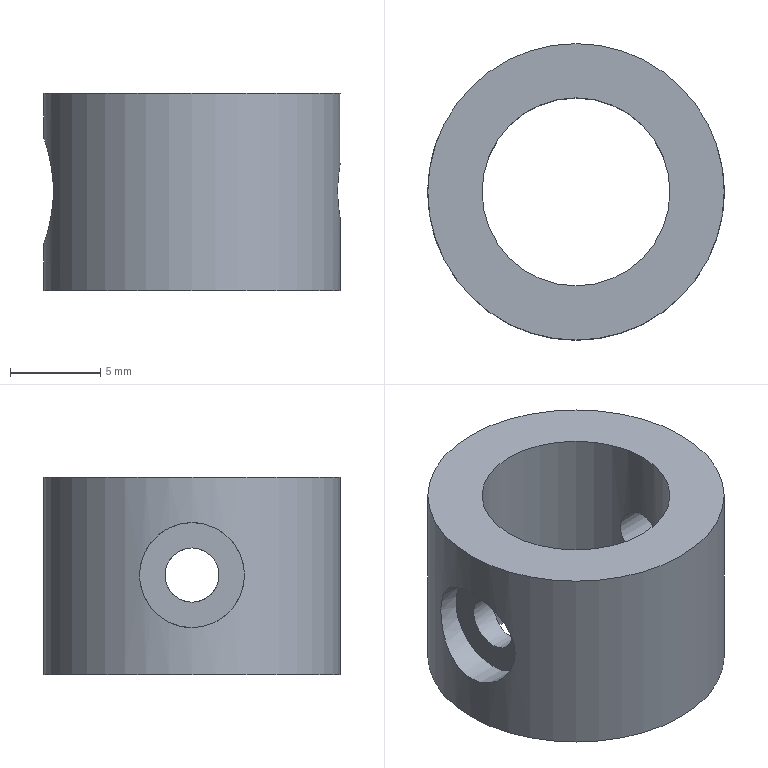Part | NX | features BREP 1, DATUM_CSYS 1 | 1 solid | 8 faces | box 16.4 x 16.4 x 10.9 mm | volume 1304 mm3 | cylinder 5 | plane 3 | commonest cylinder face diameters 3 x2 5.82 x1 10.4 x1 16.4 x1
STEP:
#1=CARTESIAN_POINT('',(23.5,0.000004761,25.));
#2=VERTEX_POINT('',#1);
#3=CARTESIAN_POINT('',(23.5,0.000004761,26.5));
#4=DIRECTION('',(1.,0.,0.));
#5=DIRECTION('',(0.,0.,-1.));
#6=AXIS2_PLACEMENT_3D('',#3,#4,#5);
#7=CIRCLE('',#6,1.5);
#8=EDGE_CURVE('',#2,#2,#7,.T.);
#9=ORIENTED_EDGE('',*,*,#8,.F.);
#10=EDGE_LOOP('',(#9));
#11=FACE_BOUND('',#10,.T.);
#12=CARTESIAN_POINT('',(24.8,0.00002708,28.));
#13=VERTEX_POINT('',#12);
#14=CARTESIAN_POINT('',(24.908,-1.176,27.675));
#15=CARTESIAN_POINT('',(24.746,0.0001692,28.163));
#16=CARTESIAN_POINT('',(24.908,1.176,27.674));
#17=CARTESIAN_POINT('',(25.078,1.662,26.502));
#18=CARTESIAN_POINT('',(24.908,1.175,25.324));
#19=CARTESIAN_POINT('',(24.746,0.0008367,24.838));
#20=CARTESIAN_POINT('',(24.908,-1.175,25.324));
#21=CARTESIAN_POINT('',(25.078,-1.662,26.5));
#22=CARTESIAN_POINT('',(24.908,-1.176,27.675));
#23=CARTESIAN_POINT('',(24.746,0.0001692,28.163));
#24=CARTESIAN_POINT('',(24.908,1.176,27.674));
#25=B_SPLINE_CURVE_WITH_KNOTS('',3,(#14,#15,#16,#17,#18,#19,#20,#21,#22,#23,#24),.UNSPECIFIED.,.T.,.F.,(1,1,1,1,1,1,1,1,1,1,1,1,1,1,1),(-0.003536,-0.002357,-0.001179,0.,0.001179,0.002357,0.003536,0.004714,0.005893,0.007071,0.00825,0.009428,0.01061,0.01179,0.01296),.UNSPECIFIED.);
#26=EDGE_CURVE('',#13,#13,#25,.T.);
#27=ORIENTED_EDGE('',*,*,#26,.F.);
#28=EDGE_LOOP('',(#27));
#29=FACE_BOUND('',#28,.T.);
#30=CARTESIAN_POINT('',(41.,0.000004761,26.5));
#31=DIRECTION('',(-1.,0.,0.));
#32=DIRECTION('',(0.,0.,-1.));
#33=AXIS2_PLACEMENT_3D('',#30,#31,#32);
#34=CYLINDRICAL_SURFACE('',#33,1.5);
#35=ADVANCED_FACE('',(#11,#29),#34,.F.);
#36=CARTESIAN_POINT('',(35.2,0.000004761,28.));
#37=VERTEX_POINT('',#36);
#38=CARTESIAN_POINT('',(35.092,1.176,27.675));
#39=CARTESIAN_POINT('',(35.254,-0.0001353,28.163));
#40=CARTESIAN_POINT('',(35.092,-1.176,27.674));
#41=CARTESIAN_POINT('',(34.923,-1.662,26.502));
#42=CARTESIAN_POINT('',(35.092,-1.175,25.324));
#43=CARTESIAN_POINT('',(35.254,-0.0008555,24.838));
#44=CARTESIAN_POINT('',(35.092,1.175,25.324));
#45=CARTESIAN_POINT('',(34.923,1.662,26.5));
#46=CARTESIAN_POINT('',(35.092,1.176,27.675));
#47=CARTESIAN_POINT('',(35.254,-0.0001353,28.163));
#48=CARTESIAN_POINT('',(35.092,-1.176,27.674));
#49=B_SPLINE_CURVE_WITH_KNOTS('',3,(#38,#39,#40,#41,#42,#43,#44,#45,#46,#47,#48),.UNSPECIFIED.,.T.,.F.,(1,1,1,1,1,1,1,1,1,1,1,1,1,1,1),(-0.003536,-0.002357,-0.001179,0.,0.001179,0.002357,0.003536,0.004714,0.005893,0.007071,0.00825,0.009428,0.01061,0.01179,0.01296),.UNSPECIFIED.);
#50=EDGE_CURVE('',#37,#37,#49,.T.);
#51=ORIENTED_EDGE('',*,*,#50,.T.);
#52=EDGE_LOOP('',(#51));
#53=FACE_BOUND('',#52,.T.);
#54=CARTESIAN_POINT('',(35.2,0.00002708,31.9));
#55=VERTEX_POINT('',#54);
#56=CARTESIAN_POINT('',(30.,0.00002708,31.9));
#57=DIRECTION('',(0.,0.,1.));
#58=DIRECTION('',(1.,0.,0.));
#59=AXIS2_PLACEMENT_3D('',#56,#57,#58);
#60=CIRCLE('',#59,5.2);
#61=EDGE_CURVE('',#55,#55,#60,.T.);
#62=ORIENTED_EDGE('',*,*,#61,.T.);
#63=EDGE_LOOP('',(#62));
#64=FACE_BOUND('',#63,.T.);
#65=CARTESIAN_POINT('',(35.2,0.00002708,21.));
#66=VERTEX_POINT('',#65);
#67=CARTESIAN_POINT('',(30.,0.00002708,21.));
#68=DIRECTION('',(0.,0.,1.));
#69=DIRECTION('',(1.,0.,0.));
#70=AXIS2_PLACEMENT_3D('',#67,#68,#69);
#71=CIRCLE('',#70,5.2);
#72=EDGE_CURVE('',#66,#66,#71,.T.);
#73=ORIENTED_EDGE('',*,*,#72,.F.);
#74=EDGE_LOOP('',(#73));
#75=FACE_BOUND('',#74,.T.);
#76=ORIENTED_EDGE('',*,*,#26,.T.);
#77=EDGE_LOOP('',(#76));
#78=FACE_BOUND('',#77,.T.);
#79=CARTESIAN_POINT('',(30.,0.00002708,31.9));
#80=DIRECTION('',(0.,0.,-1.));
#81=DIRECTION('',(1.,0.,0.));
#82=AXIS2_PLACEMENT_3D('',#79,#80,#81);
#83=CYLINDRICAL_SURFACE('',#82,5.2);
#84=ADVANCED_FACE('',(#53,#64,#75,#78),#83,.F.);
#85=ORIENTED_EDGE('',*,*,#61,.F.);
#86=EDGE_LOOP('',(#85));
#87=FACE_BOUND('',#86,.T.);
#88=CARTESIAN_POINT('',(38.2,0.00002708,31.9));
#89=VERTEX_POINT('',#88);
#90=CARTESIAN_POINT('',(30.,0.00002708,31.9));
#91=DIRECTION('',(0.,0.,1.));
#92=DIRECTION('',(1.,0.,0.));
#93=AXIS2_PLACEMENT_3D('',#90,#91,#92);
#94=CIRCLE('',#93,8.2);
#95=EDGE_CURVE('',#89,#89,#94,.T.);
#96=ORIENTED_EDGE('',*,*,#95,.T.);
#97=EDGE_LOOP('',(#96));
#98=FACE_BOUND('',#97,.T.);
#99=CARTESIAN_POINT('',(0.,0.,31.9));
#100=DIRECTION('',(0.,0.,1.));
#101=DIRECTION('',(-1.,0.,0.));
#102=AXIS2_PLACEMENT_3D('',#99,#100,#101);
#103=PLANE('',#102);
#104=ADVANCED_FACE('',(#87,#98),#103,.T.);
#105=CARTESIAN_POINT('',(38.2,0.000004761,28.));
#106=VERTEX_POINT('',#105);
#107=CARTESIAN_POINT('',(38.131,1.177,27.674));
#108=CARTESIAN_POINT('',(38.234,-0.0002671,28.163));
#109=CARTESIAN_POINT('',(38.131,-1.176,27.675));
#110=CARTESIAN_POINT('',(38.027,-1.662,26.502));
#111=CARTESIAN_POINT('',(38.131,-1.176,25.325));
#112=CARTESIAN_POINT('',(38.234,-0.0004822,24.838));
#113=CARTESIAN_POINT('',(38.132,1.174,25.323));
#114=CARTESIAN_POINT('',(38.027,1.662,26.499));
#115=CARTESIAN_POINT('',(38.131,1.177,27.674));
#116=CARTESIAN_POINT('',(38.234,-0.0002671,28.163));
#117=CARTESIAN_POINT('',(38.131,-1.176,27.675));
#118=B_SPLINE_CURVE_WITH_KNOTS('',3,(#107,#108,#109,#110,#111,#112,#113,#114,#115,#116,#117),.UNSPECIFIED.,.T.,.F.,(1,1,1,1,1,1,1,1,1,1,1,1,1,1,1),(-0.003524,-0.002349,-0.001175,0.,0.001175,0.002349,0.003524,0.004699,0.005874,0.007048,0.008223,0.009398,0.01057,0.01175,0.01292),.UNSPECIFIED.);
#119=EDGE_CURVE('',#106,#106,#118,.T.);
#120=ORIENTED_EDGE('',*,*,#119,.F.);
#121=EDGE_LOOP('',(#120));
#122=FACE_BOUND('',#121,.T.);
#123=CARTESIAN_POINT('',(38.2,0.00002708,21.));
#124=VERTEX_POINT('',#123);
#125=CARTESIAN_POINT('',(30.,0.00002708,21.));
#126=DIRECTION('',(0.,0.,1.));
#127=DIRECTION('',(1.,0.,0.));
#128=AXIS2_PLACEMENT_3D('',#125,#126,#127);
#129=CIRCLE('',#128,8.2);
#130=EDGE_CURVE('',#124,#124,#129,.T.);
#131=ORIENTED_EDGE('',*,*,#130,.T.);
#132=EDGE_LOOP('',(#131));
#133=FACE_BOUND('',#132,.T.);
#134=ORIENTED_EDGE('',*,*,#95,.F.);
#135=EDGE_LOOP('',(#134));
#136=FACE_BOUND('',#135,.T.);
#137=CARTESIAN_POINT('',(21.8,0.00002708,29.41));
#138=VERTEX_POINT('',#137);
#139=CARTESIAN_POINT('',(22.058,-2.28,28.78));
#140=CARTESIAN_POINT('',(21.671,-0.0002657,29.726));
#141=CARTESIAN_POINT('',(22.058,2.282,28.778));
#142=CARTESIAN_POINT('',(22.472,3.225,26.504));
#143=CARTESIAN_POINT('',(22.058,2.279,24.219));
#144=CARTESIAN_POINT('',(21.671,0.002094,23.276));
#145=CARTESIAN_POINT('',(22.058,-2.281,24.22));
#146=CARTESIAN_POINT('',(22.472,-3.225,26.501));
#147=CARTESIAN_POINT('',(22.058,-2.28,28.78));
#148=CARTESIAN_POINT('',(21.671,-0.0002657,29.726));
#149=CARTESIAN_POINT('',(22.058,2.282,28.778));
#150=B_SPLINE_CURVE_WITH_KNOTS('',3,(#139,#140,#141,#142,#143,#144,#145,#146,#147,#148,#149),.UNSPECIFIED.,.T.,.F.,(1,1,1,1,1,1,1,1,1,1,1,1,1,1,1),(-0.006879,-0.004586,-0.002293,0.,0.002293,0.004586,0.006879,0.009172,0.01147,0.01376,0.01605,0.01834,0.02064,0.02293,0.02522),.UNSPECIFIED.);
#151=EDGE_CURVE('',#138,#138,#150,.T.);
#152=ORIENTED_EDGE('',*,*,#151,.F.);
#153=EDGE_LOOP('',(#152));
#154=FACE_BOUND('',#153,.T.);
#155=CARTESIAN_POINT('',(30.,0.00002708,31.9));
#156=DIRECTION('',(0.,0.,-1.));
#157=DIRECTION('',(1.,0.,0.));
#158=AXIS2_PLACEMENT_3D('',#155,#156,#157);
#159=CYLINDRICAL_SURFACE('',#158,8.2);
#160=ADVANCED_FACE('',(#122,#133,#136,#154),#159,.T.);
#161=ORIENTED_EDGE('',*,*,#72,.T.);
#162=EDGE_LOOP('',(#161));
#163=FACE_BOUND('',#162,.T.);
#164=ORIENTED_EDGE('',*,*,#130,.F.);
#165=EDGE_LOOP('',(#164));
#166=FACE_BOUND('',#165,.T.);
#167=CARTESIAN_POINT('',(0.,0.,21.));
#168=DIRECTION('',(0.,0.,1.));
#169=DIRECTION('',(-1.,0.,0.));
#170=AXIS2_PLACEMENT_3D('',#167,#168,#169);
#171=PLANE('',#170);
#172=ADVANCED_FACE('',(#163,#166),#171,.F.);
#173=ORIENTED_EDGE('',*,*,#8,.T.);
#174=EDGE_LOOP('',(#173));
#175=FACE_BOUND('',#174,.T.);
#176=CARTESIAN_POINT('',(23.5,0.00001352,23.59));
#177=VERTEX_POINT('',#176);
#178=CARTESIAN_POINT('',(23.5,0.00001352,26.5));
#179=DIRECTION('',(1.,0.,0.));
#180=DIRECTION('',(0.,0.,-1.));
#181=AXIS2_PLACEMENT_3D('',#178,#179,#180);
#182=CIRCLE('',#181,2.91);
#183=EDGE_CURVE('',#177,#177,#182,.T.);
#184=ORIENTED_EDGE('',*,*,#183,.F.);
#185=EDGE_LOOP('',(#184));
#186=FACE_BOUND('',#185,.T.);
#187=CARTESIAN_POINT('',(23.5,0.,0.));
#188=DIRECTION('',(1.,0.,0.));
#189=DIRECTION('',(0.,0.,1.));
#190=AXIS2_PLACEMENT_3D('',#187,#188,#189);
#191=PLANE('',#190);
#192=ADVANCED_FACE('',(#175,#186),#191,.F.);
#193=ORIENTED_EDGE('',*,*,#183,.T.);
#194=EDGE_LOOP('',(#193));
#195=FACE_BOUND('',#194,.T.);
#196=ORIENTED_EDGE('',*,*,#151,.T.);
#197=EDGE_LOOP('',(#196));
#198=FACE_BOUND('',#197,.T.);
#199=CARTESIAN_POINT('',(41.,0.00001352,26.5));
#200=DIRECTION('',(-1.,0.,0.));
#201=DIRECTION('',(0.,0.,-1.));
#202=AXIS2_PLACEMENT_3D('',#199,#200,#201);
#203=CYLINDRICAL_SURFACE('',#202,2.91);
#204=ADVANCED_FACE('',(#195,#198),#203,.F.);
#205=ORIENTED_EDGE('',*,*,#50,.F.);
#206=EDGE_LOOP('',(#205));
#207=FACE_BOUND('',#206,.T.);
#208=ORIENTED_EDGE('',*,*,#119,.T.);
#209=EDGE_LOOP('',(#208));
#210=FACE_BOUND('',#209,.T.);
#211=CARTESIAN_POINT('',(41.,0.000004761,26.5));
#212=DIRECTION('',(-1.,0.,0.));
#213=DIRECTION('',(0.,0.,-1.));
#214=AXIS2_PLACEMENT_3D('',#211,#212,#213);
#215=CYLINDRICAL_SURFACE('',#214,1.5);
#216=ADVANCED_FACE('',(#207,#210),#215,.F.);
#217=CLOSED_SHELL('',(#35,#84,#104,#160,#172,#192,#204,#216));
#218=MANIFOLD_SOLID_BREP('',#217);
#219=(LENGTH_UNIT()NAMED_UNIT(*)SI_UNIT(.MILLI.,.METRE.));
#220=UNCERTAINTY_MEASURE_WITH_UNIT(LENGTH_MEASURE(0.0508),#219,'','');
#221=(NAMED_UNIT(*)PLANE_ANGLE_UNIT()SI_UNIT($,.RADIAN.));
#222=(NAMED_UNIT(*)SI_UNIT($,.STERADIAN.)SOLID_ANGLE_UNIT());
#223=(GEOMETRIC_REPRESENTATION_CONTEXT(3)GLOBAL_UNCERTAINTY_ASSIGNED_CONTEXT((#220))GLOBAL_UNIT_ASSIGNED_CONTEXT((#219,#221,#222))REPRESENTATION_CONTEXT('',''));
#224=ADVANCED_BREP_SHAPE_REPRESENTATION('',(#218),#223);